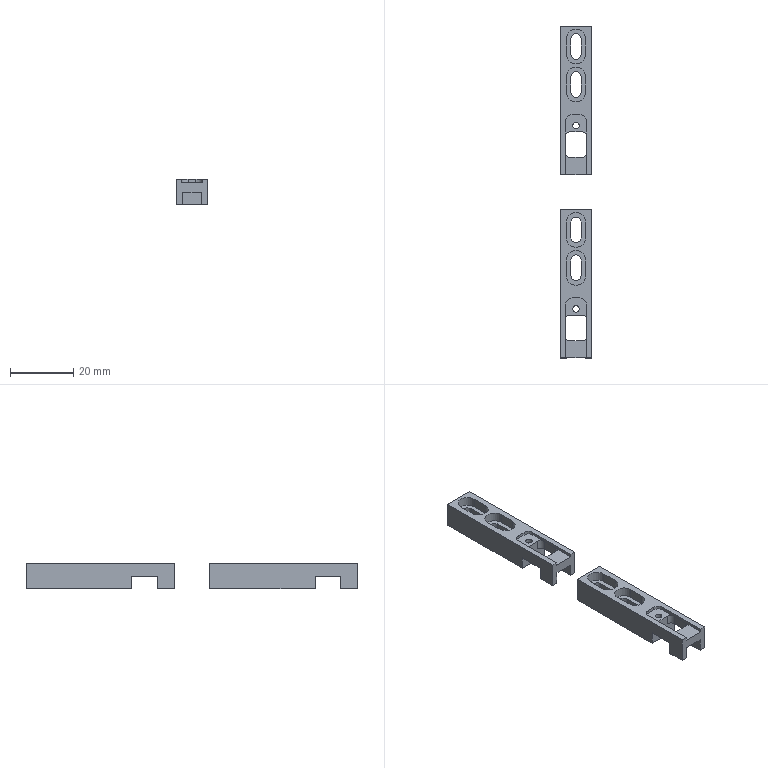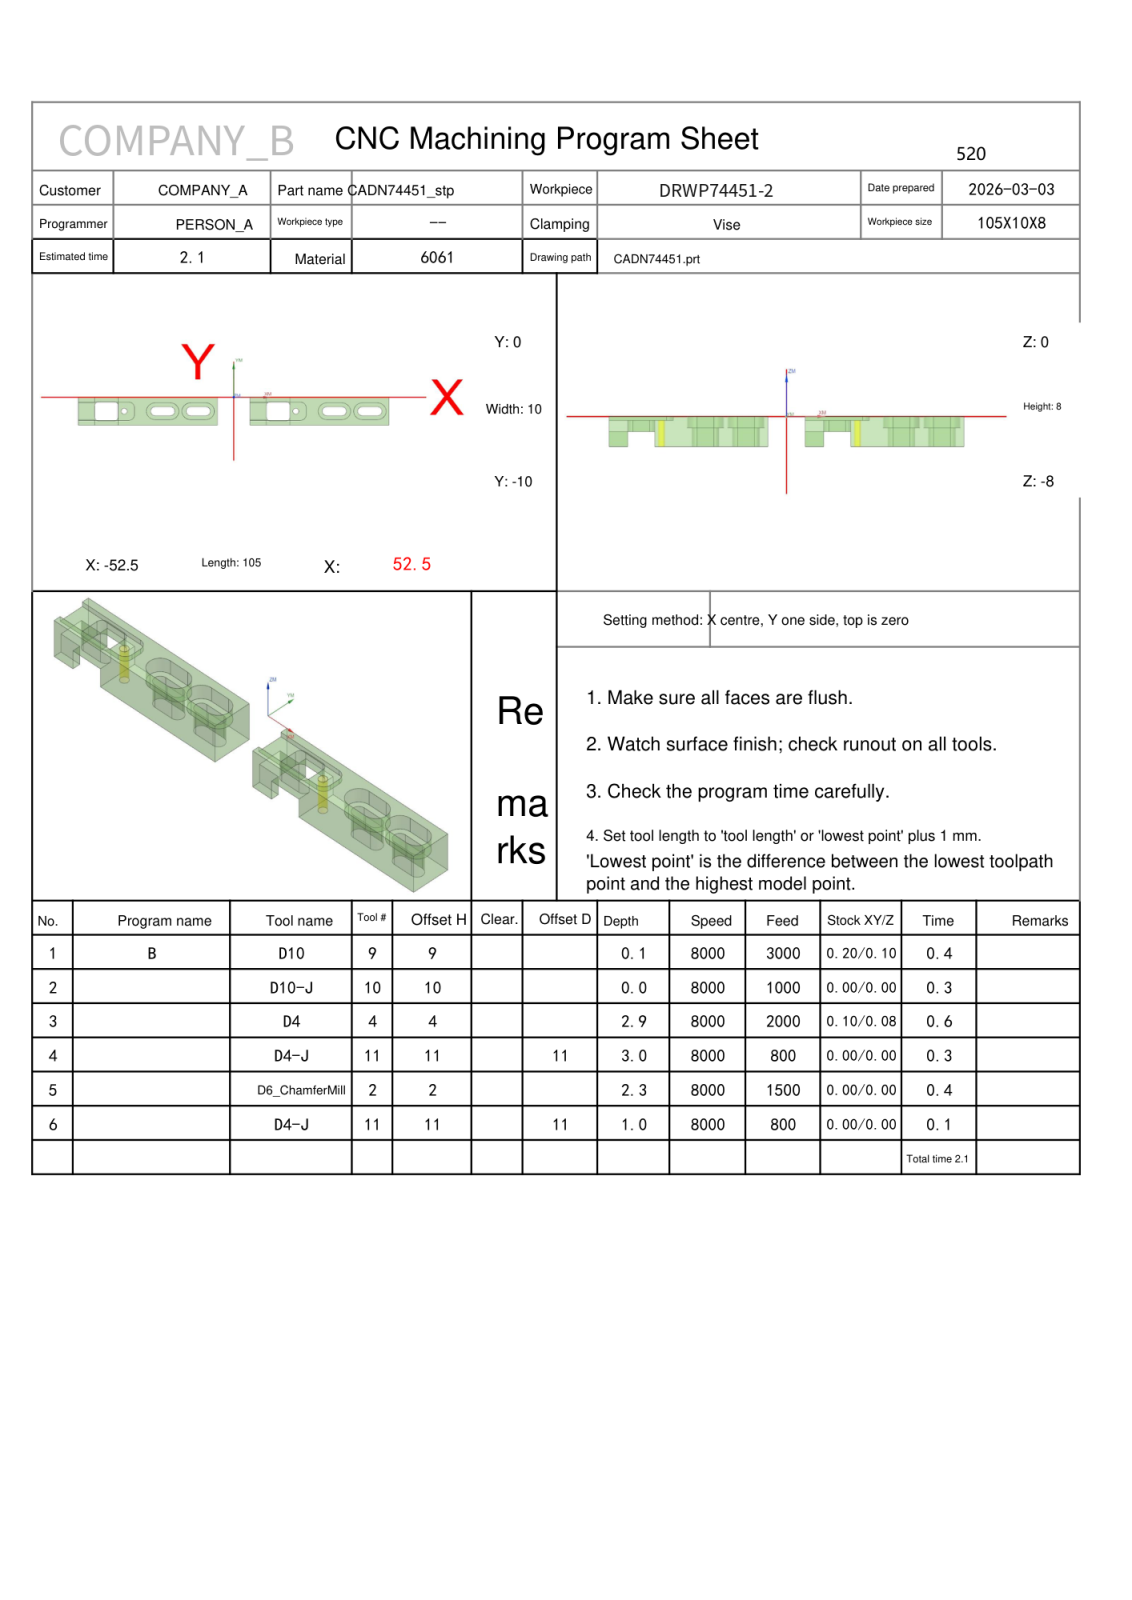NC program | NX | posted by the shop | part box 10 x 105 x 8 mm
Whole program:
%
O0001
(Machine time: 3.26 MIN)
(===Total Tool:5===)
(T9=D10     D=10.  R=0.   D-  H09 Z=0.1   )
(T10=D10-J  D=10.  R=0.   D-  H10 Z=0.    )
(T4=D4      D=4.   R=0.   D-  H04 Z=-2.94 )
(T11=D4-J   D=4.   R=0.   D11 H11 Z=-3.   )
(T2=D6_ChamferMill   D=6.   R=0.   D-  H02 Z=-2.32 )
G80 G90 G17 G49 G40
G91 G28 Z0
M01
N1 T09 M06
(D10  D=10. R=0. H=09 ce=0.20 di=0.10)
G00 G90 G54 X-69.5 Y-1.667 M03 S8000
G43 H09 Z50.
M08
Z3.525
G01 Z1.525 F3000.
X-57.5
X56.501
G02 X57.5 Y-2.666 I-.001 J-1.
G01 Y-7.333
G02 X56.5 Y-8.333 I-1. J0.0
G01 X-57.5
X-69.5
Z3.525
G00 Z5.
Y-1.667
Z3.05
G01 Z1.05
X-57.5
X56.501
G02 X57.5 Y-2.666 I-.001 J-1.
G01 Y-7.333
G02 X56.5 Y-8.333 I-1. J0.0
G01 X-57.5
X-69.5
Z3.05
G00 Z4.525
Y-1.667
Z2.575
G01 Z.575
X-57.5
X56.501
G02 X57.5 Y-2.666 I-.001 J-1.
G01 Y-7.333
G02 X56.5 Y-8.333 I-1. J0.0
G01 X-57.5
X-69.5
Z2.575
G00 Z4.05
Y-1.667
Z2.1
G01 Z.1
X-57.5
X56.501
G02 X57.5 Y-2.666 I-.001 J-1.
G01 Y-7.333
G02 X56.5 Y-8.333 I-1. J0.0
G01 X-57.5
X-69.5
Z2.1
G00 Z50.
G91 G28 Z0.0
M05
M09
G91 G28 Z0.0
M01
N2 T10 M06
(D10-J  D=10. R=0. H=10 ce=0.00 di=0.00)
G00 G90 G54 X-69.5 Y-1.667 M03 S8000
G43 H10 Z50.
M08
Z2.
G01 Z0.0 F1000.
X-57.5
X57.5
Y-8.333
X-57.5
X-69.5
Z2.
G00 Z50.
G91 G28 Z0.0
M05
M09
G91 G28 Z0.0
M01
N3 T04 M06
(D4  D=4. R=0. H=04 ce=0.10 di=0.08)
G00 G90 G54 X47.988 Y-4.1 M03 S8000
G43 H04 Z50.
M08
Z.8
G01 X43.266 Z.553 F2000.
X42.842 Y-4.342 Z.527
X42.6 Y-4.766 Z.501
Y-5.234 Z.477
X42.842 Y-5.658 Z.451
X43.266 Y-5.9 Z.426
X48.734 Z.139
X49.158 Y-5.658 Z.114
X49.4 Y-5.234 Z.088
Y-4.766 Z.063
X49.158 Y-4.342 Z.038
X48.734 Y-4.1 Z.012
X48.5 Z0.0
X43.5 Z-.094
G03 X42.6 Y-5. Z-.12 I0.0 J-.9
X43.5 Y-5.9 Z-.147 I.9 J0.0
G01 X48.5 Z-.241
G03 X49.4 Y-5. Z-.267 I0.0 J.9
X48.5 Y-4.1 Z-.294 I-.9 J0.0
G01 X43.5 Z-.388
G03 X42.6 Y-5. Z-.414 I0.0 J-.9
X43.5 Y-5.9 Z-.441 I.9 J0.0
G01 X48.5 Z-.535
G03 X49.4 Y-5. Z-.561 I0.0 J.9
X48.5 Y-4.1 Z-.588 I-.9 J0.0
G01 X43.5 Z-.682
G03 X42.6 Y-5. Z-.708 I0.0 J-.9
X43.5 Y-5.9 Z-.735 I.9 J0.0
G01 X48.5 Z-.829
G03 X49.4 Y-5. Z-.855 I0.0 J.9
X48.5 Y-4.1 Z-.882 I-.9 J0.0
G01 X43.5 Z-.976
G03 X42.6 Y-5. Z-1.002 I0.0 J-.9
X43.5 Y-5.9 Z-1.029 I.9 J0.0
G01 X48.5 Z-1.123
G03 X49.4 Y-5. Z-1.149 I0.0 J.9
X48.5 Y-4.1 Z-1.176 I-.9 J0.0
G01 X43.5 Z-1.27
G03 X42.6 Y-5. Z-1.296 I0.0 J-.9
X43.5 Y-5.9 Z-1.323 I.9 J0.0
G01 X48.5 Z-1.417
G03 X49.4 Y-5. Z-1.443 I0.0 J.9
X48.5 Y-4.1 Z-1.47 I-.9 J0.0
G01 X43.5 Z-1.564
G03 X42.6 Y-5. Z-1.59 I0.0 J-.9
X43.5 Y-5.9 Z-1.617 I.9 J0.0
G01 X48.5 Z-1.711
G03 X49.4 Y-5. Z-1.737 I0.0 J.9
X48.5 Y-4.1 Z-1.764 I-.9 J0.0
G01 X43.5 Z-1.858
G03 X42.6 Y-5. Z-1.884 I0.0 J-.9
X43.5 Y-5.9 Z-1.911 I.9 J0.0
G01 X48.5 Z-2.005
G03 X49.4 Y-5. Z-2.031 I0.0 J.9
X48.5 Y-4.1 Z-2.058 I-.9 J0.0
G01 X43.5 Z-2.152
G03 X42.6 Y-5. Z-2.178 I0.0 J-.9
X43.5 Y-5.9 Z-2.205 I.9 J0.0
G01 X48.5 Z-2.299
G03 X49.4 Y-5. Z-2.325 I0.0 J.9
X48.5 Y-4.1 Z-2.352 I-.9 J0.0
G01 X43.5 Z-2.446
G03 X42.6 Y-5. Z-2.472 I0.0 J-.9
X43.5 Y-5.9 Z-2.499 I.9 J0.0
G01 X48.5 Z-2.593
G03 X49.4 Y-5. Z-2.619 I0.0 J.9
X48.5 Y-4.1 Z-2.646 I-.9 J0.0
G01 X43.5 Z-2.74
G03 X42.6 Y-5. Z-2.766 I0.0 J-.9
X43.5 Y-5.9 Z-2.793 I.9 J0.0
G01 X48.5 Z-2.887
G03 X49.4 Y-5. Z-2.913 I0.0 J.9
X48.5 Y-4.1 Z-2.94 I-.9 J0.0
G01 X43.5
G03 X42.6 Y-5. I0.0 J-.9
X43.5 Y-5.9 I.9 J0.0
G01 X48.5
G03 X49.4 Y-5. I0.0 J.9
X48.5 Y-4.1 I-.9 J0.0
G01 X48.1
Z-2.14
G00 Z50.
X35.988
Z.8
G01 X31.266 Z.553
X30.842 Y-4.342 Z.527
X30.6 Y-4.766 Z.501
Y-5.234 Z.477
X30.842 Y-5.658 Z.451
X31.266 Y-5.9 Z.426
X36.734 Z.139
X37.158 Y-5.658 Z.114
X37.4 Y-5.234 Z.088
Y-4.766 Z.063
X37.158 Y-4.342 Z.038
X36.734 Y-4.1 Z.012
X36.5 Z0.0
X31.5 Z-.094
G03 X30.6 Y-5. Z-.12 I0.0 J-.9
X31.5 Y-5.9 Z-.147 I.9 J0.0
G01 X36.5 Z-.241
G03 X37.4 Y-5. Z-.267 I0.0 J.9
X36.5 Y-4.1 Z-.294 I-.9 J0.0
G01 X31.5 Z-.388
G03 X30.6 Y-5. Z-.414 I0.0 J-.9
X31.5 Y-5.9 Z-.441 I.9 J0.0
G01 X36.5 Z-.535
G03 X37.4 Y-5. Z-.561 I0.0 J.9
X36.5 Y-4.1 Z-.588 I-.9 J0.0
G01 X31.5 Z-.682
G03 X30.6 Y-5. Z-.708 I0.0 J-.9
X31.5 Y-5.9 Z-.735 I.9 J0.0
G01 X36.5 Z-.829
G03 X37.4 Y-5. Z-.855 I0.0 J.9
X36.5 Y-4.1 Z-.882 I-.9 J0.0
G01 X31.5 Z-.976
G03 X30.6 Y-5. Z-1.002 I0.0 J-.9
X31.5 Y-5.9 Z-1.029 I.9 J0.0
G01 X36.5 Z-1.123
G03 X37.4 Y-5. Z-1.149 I0.0 J.9
X36.5 Y-4.1 Z-1.176 I-.9 J0.0
G01 X31.5 Z-1.27
G03 X30.6 Y-5. Z-1.296 I0.0 J-.9
X31.5 Y-5.9 Z-1.323 I.9 J0.0
G01 X36.5 Z-1.417
G03 X37.4 Y-5. Z-1.443 I0.0 J.9
X36.5 Y-4.1 Z-1.47 I-.9 J0.0
G01 X31.5 Z-1.564
G03 X30.6 Y-5. Z-1.59 I0.0 J-.9
X31.5 Y-5.9 Z-1.617 I.9 J0.0
G01 X36.5 Z-1.711
G03 X37.4 Y-5. Z-1.737 I0.0 J.9
X36.5 Y-4.1 Z-1.764 I-.9 J0.0
G01 X31.5 Z-1.858
G03 X30.6 Y-5. Z-1.884 I0.0 J-.9
X31.5 Y-5.9 Z-1.911 I.9 J0.0
G01 X36.5 Z-2.005
G03 X37.4 Y-5. Z-2.031 I0.0 J.9
X36.5 Y-4.1 Z-2.058 I-.9 J0.0
G01 X31.5 Z-2.152
G03 X30.6 Y-5. Z-2.178 I0.0 J-.9
X31.5 Y-5.9 Z-2.205 I.9 J0.0
G01 X36.5 Z-2.299
G03 X37.4 Y-5. Z-2.325 I0.0 J.9
X36.5 Y-4.1 Z-2.352 I-.9 J0.0
G01 X31.5 Z-2.446
G03 X30.6 Y-5. Z-2.472 I0.0 J-.9
X31.5 Y-5.9 Z-2.499 I.9 J0.0
G01 X36.5 Z-2.593
G03 X37.4 Y-5. Z-2.619 I0.0 J.9
X36.5 Y-4.1 Z-2.646 I-.9 J0.0
G01 X31.5 Z-2.74
G03 X30.6 Y-5. Z-2.766 I0.0 J-.9
X31.5 Y-5.9 Z-2.793 I.9 J0.0
G01 X36.5 Z-2.887
G03 X37.4 Y-5. Z-2.913 I0.0 J.9
X36.5 Y-4.1 Z-2.94 I-.9 J0.0
G01 X31.5
G03 X30.6 Y-5. I0.0 J-.9
X31.5 Y-5.9 I.9 J0.0
G01 X36.5
G03 X37.4 Y-5. I0.0 J.9
X36.5 Y-4.1 I-.9 J0.0
G01 X36.1
Z-2.14
G00 Z50.
X-10.012
Z.8
G01 X-14.734 Z.553
X-15.158 Y-4.342 Z.527
X-15.4 Y-4.766 Z.501
Y-5.234 Z.477
X-15.158 Y-5.658 Z.451
X-14.734 Y-5.9 Z.426
X-9.266 Z.139
X-8.842 Y-5.658 Z.114
X-8.6 Y-5.234 Z.088
Y-4.766 Z.063
X-8.842 Y-4.342 Z.038
X-9.266 Y-4.1 Z.012
X-9.5 Z0.0
X-14.5 Z-.094
G03 X-15.4 Y-5. Z-.12 I0.0 J-.9
X-14.5 Y-5.9 Z-.147 I.9 J0.0
G01 X-9.5 Z-.241
G03 X-8.6 Y-5. Z-.267 I0.0 J.9
X-9.5 Y-4.1 Z-.294 I-.9 J0.0
G01 X-14.5 Z-.388
G03 X-15.4 Y-5. Z-.414 I0.0 J-.9
X-14.5 Y-5.9 Z-.441 I.9 J0.0
G01 X-9.5 Z-.535
G03 X-8.6 Y-5. Z-.561 I0.0 J.9
X-9.5 Y-4.1 Z-.588 I-.9 J0.0
G01 X-14.5 Z-.682
G03 X-15.4 Y-5. Z-.708 I0.0 J-.9
X-14.5 Y-5.9 Z-.735 I.9 J0.0
G01 X-9.5 Z-.829
G03 X-8.6 Y-5. Z-.855 I0.0 J.9
X-9.5 Y-4.1 Z-.882 I-.9 J0.0
G01 X-14.5 Z-.976
G03 X-15.4 Y-5. Z-1.002 I0.0 J-.9
X-14.5 Y-5.9 Z-1.029 I.9 J0.0
G01 X-9.5 Z-1.123
G03 X-8.6 Y-5. Z-1.149 I0.0 J.9
X-9.5 Y-4.1 Z-1.176 I-.9 J0.0
G01 X-14.5 Z-1.27
G03 X-15.4 Y-5. Z-1.296 I0.0 J-.9
X-14.5 Y-5.9 Z-1.323 I.9 J0.0
G01 X-9.5 Z-1.417
G03 X-8.6 Y-5. Z-1.443 I0.0 J.9
X-9.5 Y-4.1 Z-1.47 I-.9 J0.0
G01 X-14.5 Z-1.564
G03 X-15.4 Y-5. Z-1.59 I0.0 J-.9
X-14.5 Y-5.9 Z-1.617 I.9 J0.0
G01 X-9.5 Z-1.711
G03 X-8.6 Y-5. Z-1.737 I0.0 J.9
X-9.5 Y-4.1 Z-1.764 I-.9 J0.0
G01 X-14.5 Z-1.858
G03 X-15.4 Y-5. Z-1.884 I0.0 J-.9
X-14.5 Y-5.9 Z-1.911 I.9 J0.0
G01 X-9.5 Z-2.005
G03 X-8.6 Y-5. Z-2.031 I0.0 J.9
X-9.5 Y-4.1 Z-2.058 I-.9 J0.0
G01 X-14.5 Z-2.152
G03 X-15.4 Y-5. Z-2.178 I0.0 J-.9
X-14.5 Y-5.9 Z-2.205 I.9 J0.0
G01 X-9.5 Z-2.299
G03 X-8.6 Y-5. Z-2.325 I0.0 J.9
X-9.5 Y-4.1 Z-2.352 I-.9 J0.0
G01 X-14.5 Z-2.446
G03 X-15.4 Y-5. Z-2.472 I0.0 J-.9
X-14.5 Y-5.9 Z-2.499 I.9 J0.0
G01 X-9.5 Z-2.593
G03 X-8.6 Y-5. Z-2.619 I0.0 J.9
X-9.5 Y-4.1 Z-2.646 I-.9 J0.0
G01 X-14.5 Z-2.74
G03 X-15.4 Y-5. Z-2.766 I0.0 J-.9
X-14.5 Y-5.9 Z-2.793 I.9 J0.0
G01 X-9.5 Z-2.887
G03 X-8.6 Y-5. Z-2.913 I0.0 J.9
X-9.5 Y-4.1 Z-2.94 I-.9 J0.0
G01 X-14.5
G03 X-15.4 Y-5. I0.0 J-.9
X-14.5 Y-5.9 I.9 J0.0
G01 X-9.5
G03 X-8.6 Y-5. I0.0 J.9
X-9.5 Y-4.1 I-.9 J0.0
G01 X-9.9
Z-2.14
G00 Z50.
X-22.012
Z.8
G01 X-26.734 Z.553
X-27.158 Y-4.342 Z.527
X-27.4 Y-4.766 Z.501
Y-5.234 Z.477
X-27.158 Y-5.658 Z.451
X-26.734 Y-5.9 Z.426
X-21.266 Z.139
X-20.842 Y-5.658 Z.114
X-20.6 Y-5.234 Z.088
Y-4.766 Z.063
X-20.842 Y-4.342 Z.038
X-21.266 Y-4.1 Z.012
X-21.5 Z0.0
X-26.5 Z-.094
G03 X-27.4 Y-5. Z-.12 I0.0 J-.9
X-26.5 Y-5.9 Z-.147 I.9 J0.0
G01 X-21.5 Z-.241
G03 X-20.6 Y-5. Z-.267 I0.0 J.9
X-21.5 Y-4.1 Z-.294 I-.9 J0.0
G01 X-26.5 Z-.388
G03 X-27.4 Y-5. Z-.414 I0.0 J-.9
X-26.5 Y-5.9 Z-.441 I.9 J0.0
G01 X-21.5 Z-.535
G03 X-20.6 Y-5. Z-.561 I0.0 J.9
X-21.5 Y-4.1 Z-.588 I-.9 J0.0
G01 X-26.5 Z-.682
G03 X-27.4 Y-5. Z-.708 I0.0 J-.9
X-26.5 Y-5.9 Z-.735 I.9 J0.0
G01 X-21.5 Z-.829
G03 X-20.6 Y-5. Z-.855 I0.0 J.9
X-21.5 Y-4.1 Z-.882 I-.9 J0.0
G01 X-26.5 Z-.976
G03 X-27.4 Y-5. Z-1.002 I0.0 J-.9
X-26.5 Y-5.9 Z-1.029 I.9 J0.0
G01 X-21.5 Z-1.123
G03 X-20.6 Y-5. Z-1.149 I0.0 J.9
X-21.5 Y-4.1 Z-1.176 I-.9 J0.0
G01 X-26.5 Z-1.27
G03 X-27.4 Y-5. Z-1.296 I0.0 J-.9
X-26.5 Y-5.9 Z-1.323 I.9 J0.0
G01 X-21.5 Z-1.417
G03 X-20.6 Y-5. Z-1.443 I0.0 J.9
X-21.5 Y-4.1 Z-1.47 I-.9 J0.0
G01 X-26.5 Z-1.564
G03 X-27.4 Y-5. Z-1.59 I0.0 J-.9
X-26.5 Y-5.9 Z-1.617 I.9 J0.0
G01 X-21.5 Z-1.711
G03 X-20.6 Y-5. Z-1.737 I0.0 J.9
X-21.5 Y-4.1 Z-1.764 I-.9 J0.0
G01 X-26.5 Z-1.858
G03 X-27.4 Y-5. Z-1.884 I0.0 J-.9
X-26.5 Y-5.9 Z-1.911 I.9 J0.0
G01 X-21.5 Z-2.005
G03 X-20.6 Y-5. Z-2.031 I0.0 J.9
X-21.5 Y-4.1 Z-2.058 I-.9 J0.0
G01 X-26.5 Z-2.152
G03 X-27.4 Y-5. Z-2.178 I0.0 J-.9
X-26.5 Y-5.9 Z-2.205 I.9 J0.0
G01 X-21.5 Z-2.299
G03 X-20.6 Y-5. Z-2.325 I0.0 J.9
X-21.5 Y-4.1 Z-2.352 I-.9 J0.0
G01 X-26.5 Z-2.446
G03 X-27.4 Y-5. Z-2.472 I0.0 J-.9
X-26.5 Y-5.9 Z-2.499 I.9 J0.0
G01 X-21.5 Z-2.593
G03 X-20.6 Y-5. Z-2.619 I0.0 J.9
X-21.5 Y-4.1 Z-2.646 I-.9 J0.0
G01 X-26.5 Z-2.74
G03 X-27.4 Y-5. Z-2.766 I0.0 J-.9
X-26.5 Y-5.9 Z-2.793 I.9 J0.0
G01 X-21.5 Z-2.887
G03 X-20.6 Y-5. Z-2.913 I0.0 J.9
X-21.5 Y-4.1 Z-2.94 I-.9 J0.0
G01 X-26.5
G03 X-27.4 Y-5. I0.0 J-.9
X-26.5 Y-5.9 I.9 J0.0
G01 X-21.5
G03 X-20.6 Y-5. I0.0 J.9
X-21.5 Y-4.1 I-.9 J0.0
G01 X-21.9
Z-2.14
G00 Z50.
G00 G90 X-57.6 Y-6.15 M03 S8000
Z11.8
Z1.2
G01 Z-.3 F2000.
X-54.46
X-35.6
Y-3.85
X-54.46
X-57.6
Z1.2
G00 Y-6.15
Z.9
G01 Z-.6
X-54.46
X-35.6
Y-3.85
X-54.46
X-57.6
Z.9
G00 Y-6.15
Z.6
G01 Z-.9
X-54.46
X-35.6
Y-3.85
X-54.46
X-57.6
Z.6
G00 Z11.8
X.4 Y-6.15
Z1.2
G01 Z-.3
X3.54
X22.4
Y-3.85
X3.54
X.4
Z1.2
G00 Y-6.15
Z.9
G01 Z-.6
X3.54
X22.4
Y-3.85
X3.54
X.4
Z.9
G00 Y-6.15
Z.6
G01 Z-.9
X3.54
X22.4
Y-3.85
X3.54
X.4
Z.6
G00 Z11.8
G91 G28 Z0.0
M05
M09
G91 G28 Z0.0
M01
N4 T11 M06
(D4-J  D=4. R=0. H=11 ce=0.00 di=0.00)
G00 G90 G54 X49.465 Y-5.017 M03 S8000
G43 H11 Z50.
M08
Z.5
G01 Y-4.902 Z.494 F800.
X49.403 Y-4.645 Z.48
X49.273 Y-4.414 Z.466
X49.086 Y-4.227 Z.452
X48.855 Y-4.097 Z.438
X48.598 Y-4.035 Z.425
X43.402 Z.152
X43.145 Y-4.097 Z.138
X42.914 Y-4.227 Z.125
X42.727 Y-4.414 Z.111
X42.597 Y-4.645 Z.097
X42.535 Y-4.902 Z.083
Y-5.098 Z.073
X42.595 Y-5.349 Z.059
X42.718 Y-5.575 Z.046
X42.897 Y-5.76 Z.032
X43.118 Y-5.892 Z.019
X43.366 Y-5.961 Z.005
X43.465 Y-5.965 Z0.0
G41 D11
X43.5 Y-6.
X48.5 Z-.461
G03 X49.5 Y-5. Z-.605 I0.0 J1.
X48.5 Y-4. Z-.75 I-1. J0.0
G01 X43.5 Z-1.211
G03 X42.5 Y-5. Z-1.355 I0.0 J-1.
X43.5 Y-6. Z-1.5 I1. J0.0
G01 X48.5 Z-1.961
G03 X49.5 Y-5. Z-2.105 I0.0 J1.
X48.5 Y-4. Z-2.25 I-1. J0.0
G01 X43.5 Z-2.711
G03 X42.5 Y-5. Z-2.855 I0.0 J-1.
X43.5 Y-6. Z-3. I1. J0.0
G01 X48.5
G03 X49.5 Y-5. I0.0 J1.
X48.5 Y-4. I-1. J0.0
G01 X43.5
G03 X42.5 Y-5. I0.0 J-1.
X43.5 Y-6. I1. J0.0
G01 X43.9
X43.928 Y-5.998
X43.948 Y-5.978
X43.95 Y-5.95
G40 Y-5.9
Z-2.
G00 Z50.
X37.465 Y-5.017
Z.5
G01 Y-4.902 Z.494
X37.403 Y-4.645 Z.48
X37.273 Y-4.414 Z.466
X37.086 Y-4.227 Z.452
X36.855 Y-4.097 Z.438
X36.598 Y-4.035 Z.425
X31.402 Z.152
X31.145 Y-4.097 Z.138
X30.914 Y-4.227 Z.125
X30.727 Y-4.414 Z.111
X30.597 Y-4.645 Z.097
X30.535 Y-4.902 Z.083
Y-5.098 Z.073
X30.595 Y-5.349 Z.059
X30.718 Y-5.575 Z.046
X30.897 Y-5.76 Z.032
X31.118 Y-5.892 Z.019
X31.366 Y-5.961 Z.005
X31.465 Y-5.965 Z0.0
G41 D11
X31.5 Y-6.
X36.5 Z-.461
G03 X37.5 Y-5. Z-.605 I0.0 J1.
X36.5 Y-4. Z-.75 I-1. J0.0
G01 X31.5 Z-1.211
G03 X30.5 Y-5. Z-1.355 I0.0 J-1.
X31.5 Y-6. Z-1.5 I1. J0.0
G01 X36.5 Z-1.961
G03 X37.5 Y-5. Z-2.105 I0.0 J1.
X36.5 Y-4. Z-2.25 I-1. J0.0
G01 X31.5 Z-2.711
G03 X30.5 Y-5. Z-2.855 I0.0 J-1.
X31.5 Y-6. Z-3. I1. J0.0
G01 X36.5
G03 X37.5 Y-5. I0.0 J1.
X36.5 Y-4. I-1. J0.0
G01 X31.5
G03 X30.5 Y-5. I0.0 J-1.
X31.5 Y-6. I1. J0.0
G01 X31.9
X31.928 Y-5.998
X31.948 Y-5.978
X31.95 Y-5.95
G40 Y-5.9
Z-2.
G00 Z50.
X-8.535 Y-5.017
Z.5
G01 Y-4.902 Z.494
X-8.597 Y-4.645 Z.48
X-8.727 Y-4.414 Z.466
X-8.914 Y-4.227 Z.452
X-9.145 Y-4.097 Z.438
X-9.402 Y-4.035 Z.425
X-14.598 Z.152
X-14.855 Y-4.097 Z.138
X-15.086 Y-4.227 Z.125
X-15.273 Y-4.414 Z.111
X-15.403 Y-4.645 Z.097
X-15.465 Y-4.902 Z.083
Y-5.098 Z.073
X-15.405 Y-5.349 Z.059
X-15.282 Y-5.575 Z.046
X-15.103 Y-5.76 Z.032
X-14.882 Y-5.892 Z.019
X-14.634 Y-5.961 Z.005
X-14.535 Y-5.965 Z0.0
G41 D11
X-14.5 Y-6.
X-9.5 Z-.461
G03 X-8.5 Y-5. Z-.605 I0.0 J1.
X-9.5 Y-4. Z-.75 I-1. J0.0
G01 X-14.5 Z-1.211
G03 X-15.5 Y-5. Z-1.355 I0.0 J-1.
X-14.5 Y-6. Z-1.5 I1. J0.0
G01 X-9.5 Z-1.961
G03 X-8.5 Y-5. Z-2.105 I0.0 J1.
X-9.5 Y-4. Z-2.25 I-1. J0.0
G01 X-14.5 Z-2.711
G03 X-15.5 Y-5. Z-2.855 I0.0 J-1.
X-14.5 Y-6. Z-3. I1. J0.0
G01 X-9.5
G03 X-8.5 Y-5. I0.0 J1.
X-9.5 Y-4. I-1. J0.0
G01 X-14.5
G03 X-15.5 Y-5. I0.0 J-1.
X-14.5 Y-6. I1. J0.0
G01 X-14.1
X-14.073 Y-5.998
X-14.052 Y-5.978
X-14.05 Y-5.95
G40 Y-5.9
Z-2.
G00 Z50.
X-20.535 Y-5.017
Z.5
G01 Y-4.902 Z.494
X-20.597 Y-4.645 Z.48
X-20.727 Y-4.414 Z.466
X-20.914 Y-4.227 Z.452
X-21.145 Y-4.097 Z.438
X-21.402 Y-4.035 Z.425
X-26.598 Z.152
X-26.855 Y-4.097 Z.138
X-27.086 Y-4.227 Z.125
X-27.273 Y-4.414 Z.111
X-27.403 Y-4.645 Z.097
X-27.465 Y-4.902 Z.083
Y-5.098 Z.073
X-27.405 Y-5.349 Z.059
X-27.282 Y-5.575 Z.046
X-27.103 Y-5.76 Z.032
X-26.882 Y-5.892 Z.019
X-26.634 Y-5.961 Z.005
X-26.535 Y-5.965 Z0.0
G41 D11
X-26.5 Y-6.
X-21.5 Z-.461
G03 X-20.5 Y-5. Z-.605 I0.0 J1.
X-21.5 Y-4. Z-.75 I-1. J0.0
G01 X-26.5 Z-1.211
G03 X-27.5 Y-5. Z-1.355 I0.0 J-1.
X-26.5 Y-6. Z-1.5 I1. J0.0
G01 X-21.5 Z-1.961
G03 X-20.5 Y-5. Z-2.105 I0.0 J1.
X-21.5 Y-4. Z-2.25 I-1. J0.0
G01 X-26.5 Z-2.711
G03 X-27.5 Y-5. Z-2.855 I0.0 J-1.
X-26.5 Y-6. Z-3. I1. J0.0
G01 X-21.5
G03 X-20.5 Y-5. I0.0 J1.
X-21.5 Y-4. I-1. J0.0
G01 X-26.5
G03 X-27.5 Y-5. I0.0 J-1.
X-26.5 Y-6. I1. J0.0
G01 X-26.1
X-26.073 Y-5.998
X-26.052 Y-5.978
X-26.05 Y-5.95
G40 Y-5.9
Z-2.
G00 Z50.
G91 G28 Z0.0
M05
M09
G91 G28 Z0.0
M01
N5 T02 M06
(D6_ChamferMill  D=6. R=0. H=02 ce=0.00 di=0.00)
G00 G90 G54 X21. Y-5. M03 S8000
G43 H02 Z50.
M08
G98 G81 X21. Y-5. Z-2.325 R2. F1000.
X-37.
G80
G00 Z50.
G00 G90 X29.386 Y-10.727 M03 S6500
Z50.
Z.672
G01 Z-.7 F1500.
G03 X29.1 Y-10.527 I-1.286 J-1.532
G01 X29.054 Y-10.497
X29. Y-10.5
X5.5
X5.309 Y-10.462
X5.146 Y-10.354
X5.038 Y-10.191
X5. Y-10.
Y-8.25
X5.038 Y-8.059
X5.146 Y-7.896
X5.309 Y-7.788
X5.5 Y-7.75
X22.5
G03 X24. Y-6.25 I0.0 J1.5
G01 Y-3.75
G03 X22.5 Y-2.25 I-1.5 J0.0
G01 X5.5
X5.309 Y-2.212
X5.146 Y-2.104
X5.038 Y-1.941
X5. Y-1.75
Y0.0
X5.038 Y.191
X5.146 Y.354
X5.309 Y.462
X5.5 Y.5
X52.5
X52.691 Y.462
X52.854 Y.354
X52.962 Y.191
X53. Y0.0
Y-10.
X52.962 Y-10.191
X52.854 Y-10.354
X52.691 Y-10.462
X52.5 Y-10.5
X29.
X28.946 Y-10.497
X28.9 Y-10.527
G03 X28.614 Y-10.727 I1. J-1.732
G01 Z.672
G00 Z3.05
X33.614 Y-7.273
Z.672
G01 Z-.7
G03 X33.9 Y-7.473 I1.286 J1.532
G01 X33.946 Y-7.503
X34. Y-7.5
X36.5
G03 X39. Y-5. I0.0 J2.5
X36.5 Y-2.5 I-2.5 J0.0
G01 X31.5
G03 X29. Y-5. I0.0 J-2.5
X31.5 Y-7.5 I2.5 J0.0
G01 X34.
X34.054 Y-7.503
X34.1 Y-7.473
G03 X34.386 Y-7.273 I-1. J1.732
G01 Z.672
G00 Z10.
X46.386 Y-2.727
Z.672
G01 Z-.7
G03 X46.1 Y-2.527 I-1.286 J-1.532
G01 X46.054 Y-2.497
X46. Y-2.5
X43.5
G03 X41. Y-5. I0.0 J-2.5
X43.5 Y-7.5 I2.5 J0.0
G01 X48.5
G03 X51. Y-5. I0.0 J2.5
X48.5 Y-2.5 I-2.5 J0.0
G01 X46.
X45.946 Y-2.497
X45.9 Y-2.527
G03 X45.614 Y-2.727 I1. J-1.732
G01 Z.672
G00 Z10.
X-29.386 Y.727
Z.672
G01 Z-.7
G03 X-29.1 Y.527 I1.286 J1.532
G01 X-29.054 Y.497
X-29. Y.5
X-5.5
X-5.309 Y.462
X-5.146 Y.354
X-5.038 Y.191
X-5. Y0.0
Y-10.
X-5.038 Y-10.191
X-5.146 Y-10.354
X-5.309 Y-10.462
X-5.5 Y-10.5
X-52.5
X-52.691 Y-10.462
X-52.854 Y-10.354
X-52.962 Y-10.191
X-53. Y-10.
Y-8.25
X-52.962 Y-8.059
X-52.854 Y-7.896
X-52.691 Y-7.788
X-52.5 Y-7.75
X-35.5
G03 X-34. Y-6.25 I0.0 J1.5
G01 Y-3.75
G03 X-35.5 Y-2.25 I-1.5 J0.0
G01 X-52.5
X-52.691 Y-2.212
X-52.854 Y-2.104
X-52.962 Y-1.941
X-53. Y-1.75
Y0.0
X-52.962 Y.191
X-52.854 Y.354
X-52.691 Y.462
X-52.5 Y.5
X-29.
X-28.946 Y.497
X-28.9 Y.527
G03 X-28.614 Y.727 I-1. J1.732
G01 Z.672
G00 Z3.05
X-23.614 Y-2.727
Z.672
G01 Z-.7
G03 X-23.9 Y-2.527 I-1.286 J-1.532
G01 X-23.946 Y-2.497
X-24. Y-2.5
X-26.5
G03 X-29. Y-5. I0.0 J-2.5
X-26.5 Y-7.5 I2.5 J0.0
G01 X-21.5
G03 X-19. Y-5. I0.0 J2.5
X-21.5 Y-2.5 I-2.5 J0.0
G01 X-24.
X-24.054 Y-2.497
X-24.1 Y-2.527
G03 X-24.386 Y-2.727 I1. J-1.732
G01 Z.672
G00 Z10.
X-11.614
Z.672
G01 Z-.7
G03 X-11.9 Y-2.527 I-1.286 J-1.532
G01 X-11.946 Y-2.497
X-12. Y-2.5
X-14.5
G03 X-17. Y-5. I0.0 J-2.5
X-14.5 Y-7.5 I2.5 J0.0
G01 X-9.5
G03 X-7. Y-5. I0.0 J2.5
X-9.5 Y-2.5 I-2.5 J0.0
G01 X-12.
X-12.054 Y-2.497
X-12.1 Y-2.527
G03 X-12.386 Y-2.727 I1. J-1.732
G01 Z.672
G00 Z10.
X18.5 Y-6.563
Z2.3
G01 Z-1.7
Y-3.438
Z2.3
G00 Z10.
X5. Y-6.65
Z2.3
G01 Z-1.7
Y-3.35
Z2.3
G00 X11.5 Y-3.438
G01 Z-1.7
Y-6.563
Z2.3
G00 Z10.
X-39.5
Z2.3
G01 Z-1.7
Y-3.438
Z2.3
G00 Z10.
X-53. Y-6.65
Z2.3
G01 Z-1.7
Y-3.35
Z2.3
G00 X-46.5 Y-3.438
G01 Z-1.7
Y-6.563
Z2.3
G00 Z50.
G91 G28 Z0.0
M05
M09
G91 G28 Z0.0
M01
N6 T11 M06
(D4-J  D=4. R=0. H=11 ce=0.00 di=0.00)
G00 G90 G54 X-55.3 Y-5.25 M03 S8000
G43 H11 Z11.8
M08
Z0.0
G01 Z-1. F800.
G41 D11
Y-5.45
G03 X-54.5 Y-6.25 I.8 J0.0
G01 X-35.5
Y-3.75
X-54.5
G03 X-55.3 Y-4.55 I0.0 J-.8
G01 G40 Y-4.75
Z0.0
G00 Z3.
X2.7 Y-5.25
Z0.0
G01 Z-1.
G41 D11
Y-5.45
G03 X3.5 Y-6.25 I.8 J0.0
G01 X22.5
Y-3.75
X3.5
G03 X2.7 Y-4.55 I0.0 J-.8
G01 G40 Y-4.75
Z0.0
G00 Z11.8
M05
M09
G91 G28 Z0.0
G91 G28 Y0.0
M30
%